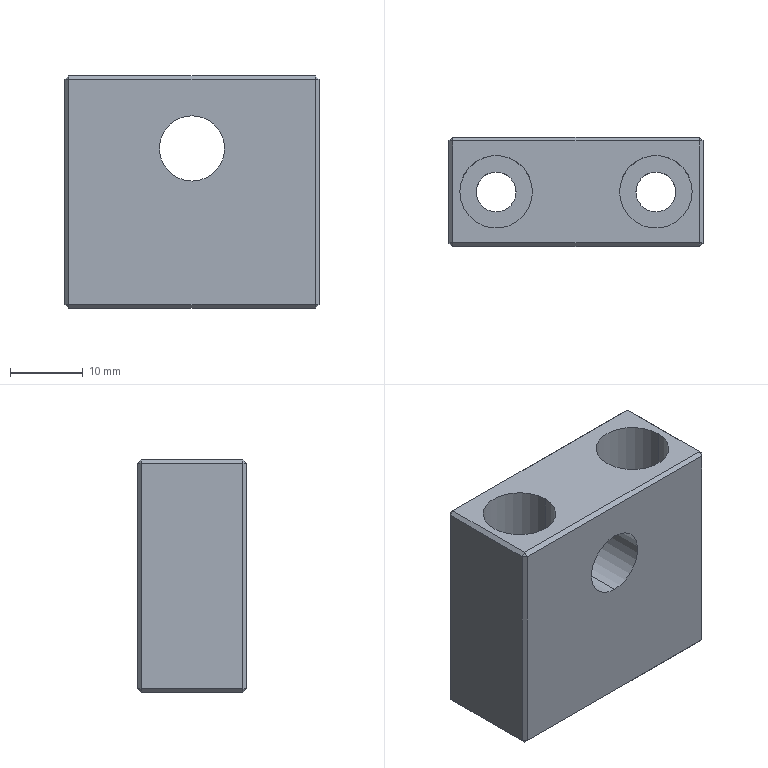Part | STEP file | ND25021-01-JDKM-11-TL | 1 solid | 38 faces | box 35 x 15 x 32 mm | volume 12641 mm3 | plane 28 | cylinder 10 | commonest cylinder face diameters 5.5 x4 10 x4 9 x2